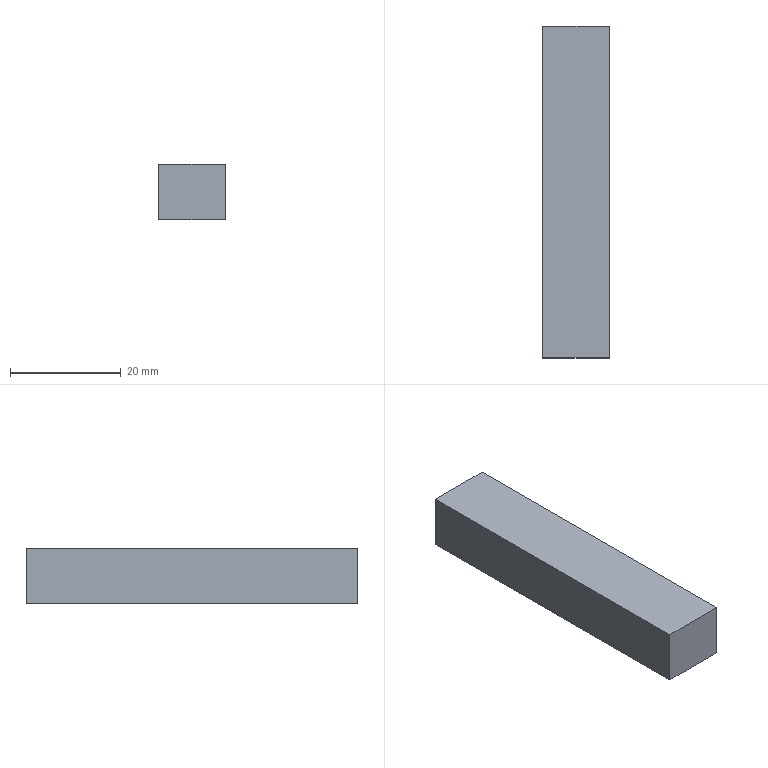Part | SolidWorks | features Extrusion 1 | 1 solid | 6 faces | box 12 x 60 x 10 mm | volume 7200 mm3 | plane 6
STEP:
#1=CARTESIAN_POINT('',(-43.665,38.769,0.));
#2=VERTEX_POINT('',#1);
#3=CARTESIAN_POINT('',(-43.665,-21.231,0.));
#4=VERTEX_POINT('',#3);
#5=CARTESIAN_POINT('',(-43.665,38.769,0.));
#6=DIRECTION('',(0.,-1.,0.));
#7=VECTOR('',#6,1000.);
#8=LINE('',#5,#7);
#9=EDGE_CURVE('',#2,#4,#8,.T.);
#10=ORIENTED_EDGE('',*,*,#9,.T.);
#11=CARTESIAN_POINT('',(-43.665,-21.231,10.));
#12=VERTEX_POINT('',#11);
#13=CARTESIAN_POINT('',(-43.665,-21.231,10.));
#14=DIRECTION('',(0.,0.,-1.));
#15=VECTOR('',#14,1000.);
#16=LINE('',#13,#15);
#17=EDGE_CURVE('',#12,#4,#16,.T.);
#18=ORIENTED_EDGE('',*,*,#17,.F.);
#19=CARTESIAN_POINT('',(-43.665,38.769,10.));
#20=VERTEX_POINT('',#19);
#21=CARTESIAN_POINT('',(-43.665,38.769,10.));
#22=DIRECTION('',(0.,-1.,0.));
#23=VECTOR('',#22,1000.);
#24=LINE('',#21,#23);
#25=EDGE_CURVE('',#20,#12,#24,.T.);
#26=ORIENTED_EDGE('',*,*,#25,.F.);
#27=CARTESIAN_POINT('',(-43.665,38.769,10.));
#28=DIRECTION('',(0.,0.,-1.));
#29=VECTOR('',#28,1000.);
#30=LINE('',#27,#29);
#31=EDGE_CURVE('',#20,#2,#30,.T.);
#32=ORIENTED_EDGE('',*,*,#31,.T.);
#33=EDGE_LOOP('',(#10,#18,#26,#32));
#34=FACE_OUTER_BOUND('',#33,.T.);
#35=CARTESIAN_POINT('',(-43.665,38.769,10.));
#36=DIRECTION('',(1.,0.,0.));
#37=DIRECTION('',(0.,1.,0.));
#38=AXIS2_PLACEMENT_3D('',#35,#36,#37);
#39=PLANE('',#38);
#40=ADVANCED_FACE('',(#34),#39,.F.);
#41=CARTESIAN_POINT('',(-31.665,-21.231,0.));
#42=VERTEX_POINT('',#41);
#43=CARTESIAN_POINT('',(-43.665,-21.231,0.));
#44=DIRECTION('',(1.,0.,0.));
#45=VECTOR('',#44,1000.);
#46=LINE('',#43,#45);
#47=EDGE_CURVE('',#4,#42,#46,.T.);
#48=ORIENTED_EDGE('',*,*,#47,.T.);
#49=CARTESIAN_POINT('',(-31.665,-21.231,10.));
#50=VERTEX_POINT('',#49);
#51=CARTESIAN_POINT('',(-31.665,-21.231,10.));
#52=DIRECTION('',(0.,0.,-1.));
#53=VECTOR('',#52,1000.);
#54=LINE('',#51,#53);
#55=EDGE_CURVE('',#50,#42,#54,.T.);
#56=ORIENTED_EDGE('',*,*,#55,.F.);
#57=CARTESIAN_POINT('',(-43.665,-21.231,10.));
#58=DIRECTION('',(1.,0.,0.));
#59=VECTOR('',#58,1000.);
#60=LINE('',#57,#59);
#61=EDGE_CURVE('',#12,#50,#60,.T.);
#62=ORIENTED_EDGE('',*,*,#61,.F.);
#63=ORIENTED_EDGE('',*,*,#17,.T.);
#64=EDGE_LOOP('',(#48,#56,#62,#63));
#65=FACE_OUTER_BOUND('',#64,.T.);
#66=CARTESIAN_POINT('',(-43.665,-21.231,10.));
#67=DIRECTION('',(0.,1.,0.));
#68=DIRECTION('',(0.,0.,1.));
#69=AXIS2_PLACEMENT_3D('',#66,#67,#68);
#70=PLANE('',#69);
#71=ADVANCED_FACE('',(#65),#70,.F.);
#72=CARTESIAN_POINT('',(-31.665,38.769,0.));
#73=VERTEX_POINT('',#72);
#74=CARTESIAN_POINT('',(-31.665,38.769,0.));
#75=DIRECTION('',(0.,1.,0.));
#76=VECTOR('',#75,1000.);
#77=LINE('',#74,#76);
#78=EDGE_CURVE('',#42,#73,#77,.T.);
#79=ORIENTED_EDGE('',*,*,#78,.T.);
#80=CARTESIAN_POINT('',(-31.665,38.769,10.));
#81=VERTEX_POINT('',#80);
#82=CARTESIAN_POINT('',(-31.665,38.769,10.));
#83=DIRECTION('',(0.,0.,-1.));
#84=VECTOR('',#83,1000.);
#85=LINE('',#82,#84);
#86=EDGE_CURVE('',#81,#73,#85,.T.);
#87=ORIENTED_EDGE('',*,*,#86,.F.);
#88=CARTESIAN_POINT('',(-31.665,38.769,10.));
#89=DIRECTION('',(0.,1.,0.));
#90=VECTOR('',#89,1000.);
#91=LINE('',#88,#90);
#92=EDGE_CURVE('',#50,#81,#91,.T.);
#93=ORIENTED_EDGE('',*,*,#92,.F.);
#94=ORIENTED_EDGE('',*,*,#55,.T.);
#95=EDGE_LOOP('',(#79,#87,#93,#94));
#96=FACE_OUTER_BOUND('',#95,.T.);
#97=CARTESIAN_POINT('',(-31.665,38.769,10.));
#98=DIRECTION('',(-1.,0.,0.));
#99=DIRECTION('',(0.,-1.,0.));
#100=AXIS2_PLACEMENT_3D('',#97,#98,#99);
#101=PLANE('',#100);
#102=ADVANCED_FACE('',(#96),#101,.F.);
#103=CARTESIAN_POINT('',(-43.665,38.769,0.));
#104=DIRECTION('',(-1.,0.,0.));
#105=VECTOR('',#104,1000.);
#106=LINE('',#103,#105);
#107=EDGE_CURVE('',#73,#2,#106,.T.);
#108=ORIENTED_EDGE('',*,*,#107,.T.);
#109=ORIENTED_EDGE('',*,*,#31,.F.);
#110=CARTESIAN_POINT('',(-43.665,38.769,10.));
#111=DIRECTION('',(-1.,0.,0.));
#112=VECTOR('',#111,1000.);
#113=LINE('',#110,#112);
#114=EDGE_CURVE('',#81,#20,#113,.T.);
#115=ORIENTED_EDGE('',*,*,#114,.F.);
#116=ORIENTED_EDGE('',*,*,#86,.T.);
#117=EDGE_LOOP('',(#108,#109,#115,#116));
#118=FACE_OUTER_BOUND('',#117,.T.);
#119=CARTESIAN_POINT('',(-43.665,38.769,10.));
#120=DIRECTION('',(0.,-1.,0.));
#121=DIRECTION('',(0.,0.,-1.));
#122=AXIS2_PLACEMENT_3D('',#119,#120,#121);
#123=PLANE('',#122);
#124=ADVANCED_FACE('',(#118),#123,.F.);
#125=ORIENTED_EDGE('',*,*,#25,.T.);
#126=ORIENTED_EDGE('',*,*,#61,.T.);
#127=ORIENTED_EDGE('',*,*,#92,.T.);
#128=ORIENTED_EDGE('',*,*,#114,.T.);
#129=EDGE_LOOP('',(#125,#126,#127,#128));
#130=FACE_OUTER_BOUND('',#129,.T.);
#131=CARTESIAN_POINT('',(0.,0.,10.));
#132=DIRECTION('',(0.,0.,1.));
#133=DIRECTION('',(1.,0.,0.));
#134=AXIS2_PLACEMENT_3D('',#131,#132,#133);
#135=PLANE('',#134);
#136=ADVANCED_FACE('',(#130),#135,.T.);
#137=ORIENTED_EDGE('',*,*,#9,.F.);
#138=ORIENTED_EDGE('',*,*,#107,.F.);
#139=ORIENTED_EDGE('',*,*,#78,.F.);
#140=ORIENTED_EDGE('',*,*,#47,.F.);
#141=EDGE_LOOP('',(#137,#138,#139,#140));
#142=FACE_OUTER_BOUND('',#141,.T.);
#143=CARTESIAN_POINT('',(0.,0.,0.));
#144=DIRECTION('',(0.,0.,1.));
#145=DIRECTION('',(1.,0.,0.));
#146=AXIS2_PLACEMENT_3D('',#143,#144,#145);
#147=PLANE('',#146);
#148=ADVANCED_FACE('',(#142),#147,.F.);
#149=CLOSED_SHELL('',(#40,#71,#102,#124,#136,#148));
#150=MANIFOLD_SOLID_BREP('',#149);
#151=CARTESIAN_POINT('',(0.,0.,0.));
#152=DIRECTION('',(0.,0.,1.));
#153=DIRECTION('',(1.,0.,0.));
#154=AXIS2_PLACEMENT_3D('',#151,#152,#153);
#155=(LENGTH_UNIT()NAMED_UNIT(*)SI_UNIT(.MILLI.,.METRE.));
#156=UNCERTAINTY_MEASURE_WITH_UNIT(LENGTH_MEASURE(0.00001),#155,'','');
#157=(NAMED_UNIT(*)PLANE_ANGLE_UNIT()SI_UNIT($,.RADIAN.));
#158=(NAMED_UNIT(*)SI_UNIT($,.STERADIAN.)SOLID_ANGLE_UNIT());
#159=(GEOMETRIC_REPRESENTATION_CONTEXT(3)GLOBAL_UNCERTAINTY_ASSIGNED_CONTEXT((#156))GLOBAL_UNIT_ASSIGNED_CONTEXT((#155,#157,#158))REPRESENTATION_CONTEXT('',''));
#160=ADVANCED_BREP_SHAPE_REPRESENTATION('',(#150,#154),#159);